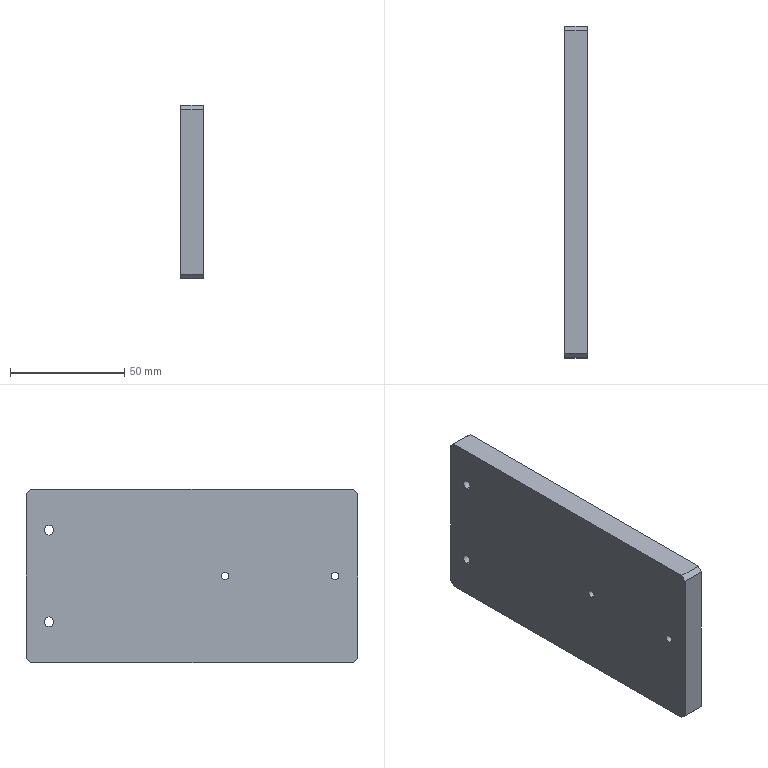Part | SolidWorks | features HoleWzd 2, Chamfer 1, Extrusion 1 | 1 solid | 18 faces | box 10 x 145 x 76 mm | volume 109672 mm3 | plane 10 | cylinder 8 | commonest cylinder face diameters 3.3 x4 4.2 x4
STEP:
#1=CARTESIAN_POINT('',(10.,-14.5,-1.65));
#2=VERTEX_POINT('',#1);
#3=CARTESIAN_POINT('',(10.,-14.5,1.65));
#4=VERTEX_POINT('',#3);
#5=CARTESIAN_POINT('',(10.,-14.5,0.));
#6=DIRECTION('',(-1.,0.,0.));
#7=DIRECTION('',(0.,0.,1.));
#8=AXIS2_PLACEMENT_3D('',#5,#6,#7);
#9=CIRCLE('',#8,1.65);
#10=EDGE_CURVE('',#2,#4,#9,.T.);
#11=ORIENTED_EDGE('',*,*,#10,.F.);
#12=CARTESIAN_POINT('',(0.,-14.5,-1.65));
#13=VERTEX_POINT('',#12);
#14=CARTESIAN_POINT('',(0.,-14.5,-1.65));
#15=DIRECTION('',(-1.,0.,0.));
#16=VECTOR('',#15,1000.);
#17=LINE('',#14,#16);
#18=EDGE_CURVE('',#2,#13,#17,.T.);
#19=ORIENTED_EDGE('',*,*,#18,.T.);
#20=CARTESIAN_POINT('',(0.,-14.5,1.65));
#21=VERTEX_POINT('',#20);
#22=CARTESIAN_POINT('',(0.,-14.5,0.));
#23=DIRECTION('',(-1.,0.,0.));
#24=DIRECTION('',(0.,0.,1.));
#25=AXIS2_PLACEMENT_3D('',#22,#23,#24);
#26=CIRCLE('',#25,1.65);
#27=EDGE_CURVE('',#13,#21,#26,.T.);
#28=ORIENTED_EDGE('',*,*,#27,.T.);
#29=CARTESIAN_POINT('',(0.,-14.5,1.65));
#30=DIRECTION('',(-1.,0.,0.));
#31=VECTOR('',#30,1000.);
#32=LINE('',#29,#31);
#33=EDGE_CURVE('',#4,#21,#32,.T.);
#34=ORIENTED_EDGE('',*,*,#33,.F.);
#35=EDGE_LOOP('',(#11,#19,#28,#34));
#36=FACE_OUTER_BOUND('',#35,.T.);
#37=CARTESIAN_POINT('',(0.,-14.5,0.));
#38=DIRECTION('',(-1.,0.,0.));
#39=DIRECTION('',(0.,0.,1.));
#40=AXIS2_PLACEMENT_3D('',#37,#38,#39);
#41=CYLINDRICAL_SURFACE('',#40,1.65);
#42=ADVANCED_FACE('',(#36),#41,.F.);
#43=CARTESIAN_POINT('',(10.,-62.5,-1.65));
#44=VERTEX_POINT('',#43);
#45=CARTESIAN_POINT('',(10.,-62.5,1.65));
#46=VERTEX_POINT('',#45);
#47=CARTESIAN_POINT('',(10.,-62.5,0.));
#48=DIRECTION('',(-1.,0.,0.));
#49=DIRECTION('',(0.,0.,1.));
#50=AXIS2_PLACEMENT_3D('',#47,#48,#49);
#51=CIRCLE('',#50,1.65);
#52=EDGE_CURVE('',#44,#46,#51,.T.);
#53=ORIENTED_EDGE('',*,*,#52,.F.);
#54=CARTESIAN_POINT('',(0.,-62.5,-1.65));
#55=VERTEX_POINT('',#54);
#56=CARTESIAN_POINT('',(0.,-62.5,-1.65));
#57=DIRECTION('',(-1.,0.,0.));
#58=VECTOR('',#57,1000.);
#59=LINE('',#56,#58);
#60=EDGE_CURVE('',#44,#55,#59,.T.);
#61=ORIENTED_EDGE('',*,*,#60,.T.);
#62=CARTESIAN_POINT('',(0.,-62.5,1.65));
#63=VERTEX_POINT('',#62);
#64=CARTESIAN_POINT('',(0.,-62.5,0.));
#65=DIRECTION('',(-1.,0.,0.));
#66=DIRECTION('',(0.,0.,1.));
#67=AXIS2_PLACEMENT_3D('',#64,#65,#66);
#68=CIRCLE('',#67,1.65);
#69=EDGE_CURVE('',#55,#63,#68,.T.);
#70=ORIENTED_EDGE('',*,*,#69,.T.);
#71=CARTESIAN_POINT('',(0.,-62.5,1.65));
#72=DIRECTION('',(-1.,0.,0.));
#73=VECTOR('',#72,1000.);
#74=LINE('',#71,#73);
#75=EDGE_CURVE('',#46,#63,#74,.T.);
#76=ORIENTED_EDGE('',*,*,#75,.F.);
#77=EDGE_LOOP('',(#53,#61,#70,#76));
#78=FACE_OUTER_BOUND('',#77,.T.);
#79=CARTESIAN_POINT('',(0.,-62.5,0.));
#80=DIRECTION('',(-1.,0.,0.));
#81=DIRECTION('',(0.,0.,1.));
#82=AXIS2_PLACEMENT_3D('',#79,#80,#81);
#83=CYLINDRICAL_SURFACE('',#82,1.65);
#84=ADVANCED_FACE('',(#78),#83,.F.);
#85=CARTESIAN_POINT('',(10.,62.5,17.9));
#86=VERTEX_POINT('',#85);
#87=CARTESIAN_POINT('',(10.,62.5,22.1));
#88=VERTEX_POINT('',#87);
#89=CARTESIAN_POINT('',(10.,62.5,20.));
#90=DIRECTION('',(-1.,0.,0.));
#91=DIRECTION('',(0.,0.,1.));
#92=AXIS2_PLACEMENT_3D('',#89,#90,#91);
#93=CIRCLE('',#92,2.1);
#94=EDGE_CURVE('',#86,#88,#93,.T.);
#95=ORIENTED_EDGE('',*,*,#94,.F.);
#96=CARTESIAN_POINT('',(0.,62.5,17.9));
#97=VERTEX_POINT('',#96);
#98=CARTESIAN_POINT('',(0.,62.5,17.9));
#99=DIRECTION('',(-1.,0.,0.));
#100=VECTOR('',#99,1000.);
#101=LINE('',#98,#100);
#102=EDGE_CURVE('',#86,#97,#101,.T.);
#103=ORIENTED_EDGE('',*,*,#102,.T.);
#104=CARTESIAN_POINT('',(0.,62.5,22.1));
#105=VERTEX_POINT('',#104);
#106=CARTESIAN_POINT('',(0.,62.5,20.));
#107=DIRECTION('',(-1.,0.,0.));
#108=DIRECTION('',(0.,0.,1.));
#109=AXIS2_PLACEMENT_3D('',#106,#107,#108);
#110=CIRCLE('',#109,2.1);
#111=EDGE_CURVE('',#97,#105,#110,.T.);
#112=ORIENTED_EDGE('',*,*,#111,.T.);
#113=CARTESIAN_POINT('',(0.,62.5,22.1));
#114=DIRECTION('',(-1.,0.,0.));
#115=VECTOR('',#114,1000.);
#116=LINE('',#113,#115);
#117=EDGE_CURVE('',#88,#105,#116,.T.);
#118=ORIENTED_EDGE('',*,*,#117,.F.);
#119=EDGE_LOOP('',(#95,#103,#112,#118));
#120=FACE_OUTER_BOUND('',#119,.T.);
#121=CARTESIAN_POINT('',(0.,62.5,20.));
#122=DIRECTION('',(-1.,0.,0.));
#123=DIRECTION('',(0.,0.,1.));
#124=AXIS2_PLACEMENT_3D('',#121,#122,#123);
#125=CYLINDRICAL_SURFACE('',#124,2.1);
#126=ADVANCED_FACE('',(#120),#125,.F.);
#127=CARTESIAN_POINT('',(10.,62.5,-22.1));
#128=VERTEX_POINT('',#127);
#129=CARTESIAN_POINT('',(10.,62.5,-17.9));
#130=VERTEX_POINT('',#129);
#131=CARTESIAN_POINT('',(10.,62.5,-20.));
#132=DIRECTION('',(-1.,0.,0.));
#133=DIRECTION('',(0.,0.,1.));
#134=AXIS2_PLACEMENT_3D('',#131,#132,#133);
#135=CIRCLE('',#134,2.1);
#136=EDGE_CURVE('',#128,#130,#135,.T.);
#137=ORIENTED_EDGE('',*,*,#136,.F.);
#138=CARTESIAN_POINT('',(0.,62.5,-22.1));
#139=VERTEX_POINT('',#138);
#140=CARTESIAN_POINT('',(0.,62.5,-22.1));
#141=DIRECTION('',(-1.,0.,0.));
#142=VECTOR('',#141,1000.);
#143=LINE('',#140,#142);
#144=EDGE_CURVE('',#128,#139,#143,.T.);
#145=ORIENTED_EDGE('',*,*,#144,.T.);
#146=CARTESIAN_POINT('',(0.,62.5,-17.9));
#147=VERTEX_POINT('',#146);
#148=CARTESIAN_POINT('',(0.,62.5,-20.));
#149=DIRECTION('',(-1.,0.,0.));
#150=DIRECTION('',(0.,0.,1.));
#151=AXIS2_PLACEMENT_3D('',#148,#149,#150);
#152=CIRCLE('',#151,2.1);
#153=EDGE_CURVE('',#139,#147,#152,.T.);
#154=ORIENTED_EDGE('',*,*,#153,.T.);
#155=CARTESIAN_POINT('',(0.,62.5,-17.9));
#156=DIRECTION('',(-1.,0.,0.));
#157=VECTOR('',#156,1000.);
#158=LINE('',#155,#157);
#159=EDGE_CURVE('',#130,#147,#158,.T.);
#160=ORIENTED_EDGE('',*,*,#159,.F.);
#161=EDGE_LOOP('',(#137,#145,#154,#160));
#162=FACE_OUTER_BOUND('',#161,.T.);
#163=CARTESIAN_POINT('',(0.,62.5,-20.));
#164=DIRECTION('',(-1.,0.,0.));
#165=DIRECTION('',(0.,0.,1.));
#166=AXIS2_PLACEMENT_3D('',#163,#164,#165);
#167=CYLINDRICAL_SURFACE('',#166,2.1);
#168=ADVANCED_FACE('',(#162),#167,.F.);
#169=CARTESIAN_POINT('',(10.,-70.5,-38.));
#170=VERTEX_POINT('',#169);
#171=CARTESIAN_POINT('',(10.,70.5,-38.));
#172=VERTEX_POINT('',#171);
#173=CARTESIAN_POINT('',(10.,72.5,-38.));
#174=DIRECTION('',(0.,1.,0.));
#175=VECTOR('',#174,1000.);
#176=LINE('',#173,#175);
#177=EDGE_CURVE('',#170,#172,#176,.T.);
#178=ORIENTED_EDGE('',*,*,#177,.F.);
#179=CARTESIAN_POINT('',(0.,-70.5,-38.));
#180=VERTEX_POINT('',#179);
#181=CARTESIAN_POINT('',(10.,-70.5,-38.));
#182=DIRECTION('',(-1.,0.,0.));
#183=VECTOR('',#182,1000.);
#184=LINE('',#181,#183);
#185=EDGE_CURVE('',#170,#180,#184,.T.);
#186=ORIENTED_EDGE('',*,*,#185,.T.);
#187=CARTESIAN_POINT('',(0.,70.5,-38.));
#188=VERTEX_POINT('',#187);
#189=CARTESIAN_POINT('',(0.,72.5,-38.));
#190=DIRECTION('',(0.,1.,0.));
#191=VECTOR('',#190,1000.);
#192=LINE('',#189,#191);
#193=EDGE_CURVE('',#180,#188,#192,.T.);
#194=ORIENTED_EDGE('',*,*,#193,.T.);
#195=CARTESIAN_POINT('',(10.,70.5,-38.));
#196=DIRECTION('',(1.,0.,0.));
#197=VECTOR('',#196,1000.);
#198=LINE('',#195,#197);
#199=EDGE_CURVE('',#188,#172,#198,.T.);
#200=ORIENTED_EDGE('',*,*,#199,.T.);
#201=EDGE_LOOP('',(#178,#186,#194,#200));
#202=FACE_OUTER_BOUND('',#201,.T.);
#203=CARTESIAN_POINT('',(10.,72.5,-38.));
#204=DIRECTION('',(0.,0.,1.));
#205=DIRECTION('',(0.,-1.,0.));
#206=AXIS2_PLACEMENT_3D('',#203,#204,#205);
#207=PLANE('',#206);
#208=ADVANCED_FACE('',(#202),#207,.F.);
#209=CARTESIAN_POINT('',(0.,72.5,-36.));
#210=VERTEX_POINT('',#209);
#211=CARTESIAN_POINT('',(0.,72.5,36.));
#212=VERTEX_POINT('',#211);
#213=CARTESIAN_POINT('',(0.,72.5,38.));
#214=DIRECTION('',(0.,0.,1.));
#215=VECTOR('',#214,1000.);
#216=LINE('',#213,#215);
#217=EDGE_CURVE('',#210,#212,#216,.T.);
#218=ORIENTED_EDGE('',*,*,#217,.T.);
#219=CARTESIAN_POINT('',(10.,72.5,36.));
#220=VERTEX_POINT('',#219);
#221=CARTESIAN_POINT('',(10.,72.5,36.));
#222=DIRECTION('',(1.,0.,0.));
#223=VECTOR('',#222,1000.);
#224=LINE('',#221,#223);
#225=EDGE_CURVE('',#212,#220,#224,.T.);
#226=ORIENTED_EDGE('',*,*,#225,.T.);
#227=CARTESIAN_POINT('',(10.,72.5,-36.));
#228=VERTEX_POINT('',#227);
#229=CARTESIAN_POINT('',(10.,72.5,38.));
#230=DIRECTION('',(0.,0.,1.));
#231=VECTOR('',#230,1000.);
#232=LINE('',#229,#231);
#233=EDGE_CURVE('',#228,#220,#232,.T.);
#234=ORIENTED_EDGE('',*,*,#233,.F.);
#235=CARTESIAN_POINT('',(10.,72.5,-36.));
#236=DIRECTION('',(-1.,0.,0.));
#237=VECTOR('',#236,1000.);
#238=LINE('',#235,#237);
#239=EDGE_CURVE('',#228,#210,#238,.T.);
#240=ORIENTED_EDGE('',*,*,#239,.T.);
#241=EDGE_LOOP('',(#218,#226,#234,#240));
#242=FACE_OUTER_BOUND('',#241,.T.);
#243=CARTESIAN_POINT('',(10.,72.5,38.));
#244=DIRECTION('',(0.,-1.,0.));
#245=DIRECTION('',(0.,0.,-1.));
#246=AXIS2_PLACEMENT_3D('',#243,#244,#245);
#247=PLANE('',#246);
#248=ADVANCED_FACE('',(#242),#247,.F.);
#249=CARTESIAN_POINT('',(0.,70.5,38.));
#250=VERTEX_POINT('',#249);
#251=CARTESIAN_POINT('',(0.,-70.5,38.));
#252=VERTEX_POINT('',#251);
#253=CARTESIAN_POINT('',(0.,72.5,38.));
#254=DIRECTION('',(0.,-1.,0.));
#255=VECTOR('',#254,1000.);
#256=LINE('',#253,#255);
#257=EDGE_CURVE('',#250,#252,#256,.T.);
#258=ORIENTED_EDGE('',*,*,#257,.T.);
#259=CARTESIAN_POINT('',(10.,-70.5,38.));
#260=VERTEX_POINT('',#259);
#261=CARTESIAN_POINT('',(10.,-70.5,38.));
#262=DIRECTION('',(1.,0.,0.));
#263=VECTOR('',#262,1000.);
#264=LINE('',#261,#263);
#265=EDGE_CURVE('',#252,#260,#264,.T.);
#266=ORIENTED_EDGE('',*,*,#265,.T.);
#267=CARTESIAN_POINT('',(10.,70.5,38.));
#268=VERTEX_POINT('',#267);
#269=CARTESIAN_POINT('',(10.,72.5,38.));
#270=DIRECTION('',(0.,-1.,0.));
#271=VECTOR('',#270,1000.);
#272=LINE('',#269,#271);
#273=EDGE_CURVE('',#268,#260,#272,.T.);
#274=ORIENTED_EDGE('',*,*,#273,.F.);
#275=CARTESIAN_POINT('',(10.,70.5,38.));
#276=DIRECTION('',(-1.,0.,0.));
#277=VECTOR('',#276,1000.);
#278=LINE('',#275,#277);
#279=EDGE_CURVE('',#268,#250,#278,.T.);
#280=ORIENTED_EDGE('',*,*,#279,.T.);
#281=EDGE_LOOP('',(#258,#266,#274,#280));
#282=FACE_OUTER_BOUND('',#281,.T.);
#283=CARTESIAN_POINT('',(10.,72.5,38.));
#284=DIRECTION('',(0.,0.,-1.));
#285=DIRECTION('',(0.,1.,0.));
#286=AXIS2_PLACEMENT_3D('',#283,#284,#285);
#287=PLANE('',#286);
#288=ADVANCED_FACE('',(#282),#287,.F.);
#289=CARTESIAN_POINT('',(0.,-72.5,36.));
#290=VERTEX_POINT('',#289);
#291=CARTESIAN_POINT('',(0.,-72.5,-36.));
#292=VERTEX_POINT('',#291);
#293=CARTESIAN_POINT('',(0.,-72.5,38.));
#294=DIRECTION('',(0.,0.,-1.));
#295=VECTOR('',#294,1000.);
#296=LINE('',#293,#295);
#297=EDGE_CURVE('',#290,#292,#296,.T.);
#298=ORIENTED_EDGE('',*,*,#297,.T.);
#299=CARTESIAN_POINT('',(10.,-72.5,-36.));
#300=VERTEX_POINT('',#299);
#301=CARTESIAN_POINT('',(10.,-72.5,-36.));
#302=DIRECTION('',(1.,0.,0.));
#303=VECTOR('',#302,1000.);
#304=LINE('',#301,#303);
#305=EDGE_CURVE('',#292,#300,#304,.T.);
#306=ORIENTED_EDGE('',*,*,#305,.T.);
#307=CARTESIAN_POINT('',(10.,-72.5,36.));
#308=VERTEX_POINT('',#307);
#309=CARTESIAN_POINT('',(10.,-72.5,38.));
#310=DIRECTION('',(0.,0.,-1.));
#311=VECTOR('',#310,1000.);
#312=LINE('',#309,#311);
#313=EDGE_CURVE('',#308,#300,#312,.T.);
#314=ORIENTED_EDGE('',*,*,#313,.F.);
#315=CARTESIAN_POINT('',(10.,-72.5,36.));
#316=DIRECTION('',(-1.,0.,0.));
#317=VECTOR('',#316,1000.);
#318=LINE('',#315,#317);
#319=EDGE_CURVE('',#308,#290,#318,.T.);
#320=ORIENTED_EDGE('',*,*,#319,.T.);
#321=EDGE_LOOP('',(#298,#306,#314,#320));
#322=FACE_OUTER_BOUND('',#321,.T.);
#323=CARTESIAN_POINT('',(10.,-72.5,38.));
#324=DIRECTION('',(0.,1.,0.));
#325=DIRECTION('',(0.,0.,1.));
#326=AXIS2_PLACEMENT_3D('',#323,#324,#325);
#327=PLANE('',#326);
#328=ADVANCED_FACE('',(#322),#327,.F.);
#329=CARTESIAN_POINT('',(10.,-14.5,0.));
#330=DIRECTION('',(-1.,0.,0.));
#331=DIRECTION('',(0.,0.,1.));
#332=AXIS2_PLACEMENT_3D('',#329,#330,#331);
#333=CIRCLE('',#332,1.65);
#334=EDGE_CURVE('',#4,#2,#333,.T.);
#335=ORIENTED_EDGE('',*,*,#334,.T.);
#336=ORIENTED_EDGE('',*,*,#10,.T.);
#337=EDGE_LOOP('',(#335,#336));
#338=FACE_BOUND('',#337,.T.);
#339=CARTESIAN_POINT('',(10.,-62.5,0.));
#340=DIRECTION('',(-1.,0.,0.));
#341=DIRECTION('',(0.,0.,1.));
#342=AXIS2_PLACEMENT_3D('',#339,#340,#341);
#343=CIRCLE('',#342,1.65);
#344=EDGE_CURVE('',#46,#44,#343,.T.);
#345=ORIENTED_EDGE('',*,*,#344,.T.);
#346=ORIENTED_EDGE('',*,*,#52,.T.);
#347=EDGE_LOOP('',(#345,#346));
#348=FACE_BOUND('',#347,.T.);
#349=CARTESIAN_POINT('',(10.,62.5,20.));
#350=DIRECTION('',(-1.,0.,0.));
#351=DIRECTION('',(0.,0.,1.));
#352=AXIS2_PLACEMENT_3D('',#349,#350,#351);
#353=CIRCLE('',#352,2.1);
#354=EDGE_CURVE('',#88,#86,#353,.T.);
#355=ORIENTED_EDGE('',*,*,#354,.T.);
#356=ORIENTED_EDGE('',*,*,#94,.T.);
#357=EDGE_LOOP('',(#355,#356));
#358=FACE_BOUND('',#357,.T.);
#359=CARTESIAN_POINT('',(10.,62.5,-20.));
#360=DIRECTION('',(-1.,0.,0.));
#361=DIRECTION('',(0.,0.,1.));
#362=AXIS2_PLACEMENT_3D('',#359,#360,#361);
#363=CIRCLE('',#362,2.1);
#364=EDGE_CURVE('',#130,#128,#363,.T.);
#365=ORIENTED_EDGE('',*,*,#364,.T.);
#366=ORIENTED_EDGE('',*,*,#136,.T.);
#367=EDGE_LOOP('',(#365,#366));
#368=FACE_BOUND('',#367,.T.);
#369=ORIENTED_EDGE('',*,*,#313,.T.);
#370=CARTESIAN_POINT('',(10.,-54.25,-54.25));
#371=DIRECTION('',(0.,0.7071,-0.7071));
#372=VECTOR('',#371,1000.);
#373=LINE('',#370,#372);
#374=EDGE_CURVE('',#300,#170,#373,.T.);
#375=ORIENTED_EDGE('',*,*,#374,.T.);
#376=ORIENTED_EDGE('',*,*,#177,.T.);
#377=CARTESIAN_POINT('',(10.,54.25,-54.25));
#378=DIRECTION('',(0.,0.7071,0.7071));
#379=VECTOR('',#378,1000.);
#380=LINE('',#377,#379);
#381=EDGE_CURVE('',#172,#228,#380,.T.);
#382=ORIENTED_EDGE('',*,*,#381,.T.);
#383=ORIENTED_EDGE('',*,*,#233,.T.);
#384=CARTESIAN_POINT('',(10.,54.25,54.25));
#385=DIRECTION('',(0.,-0.7071,0.7071));
#386=VECTOR('',#385,1000.);
#387=LINE('',#384,#386);
#388=EDGE_CURVE('',#220,#268,#387,.T.);
#389=ORIENTED_EDGE('',*,*,#388,.T.);
#390=ORIENTED_EDGE('',*,*,#273,.T.);
#391=CARTESIAN_POINT('',(10.,-54.25,54.25));
#392=DIRECTION('',(0.,-0.7071,-0.7071));
#393=VECTOR('',#392,1000.);
#394=LINE('',#391,#393);
#395=EDGE_CURVE('',#260,#308,#394,.T.);
#396=ORIENTED_EDGE('',*,*,#395,.T.);
#397=EDGE_LOOP('',(#369,#375,#376,#382,#383,#389,#390,#396));
#398=FACE_OUTER_BOUND('',#397,.T.);
#399=CARTESIAN_POINT('',(10.,0.,0.));
#400=DIRECTION('',(1.,0.,0.));
#401=DIRECTION('',(0.,0.,-1.));
#402=AXIS2_PLACEMENT_3D('',#399,#400,#401);
#403=PLANE('',#402);
#404=ADVANCED_FACE('',(#338,#348,#358,#368,#398),#403,.T.);
#405=CARTESIAN_POINT('',(0.,-14.5,0.));
#406=DIRECTION('',(-1.,0.,0.));
#407=DIRECTION('',(0.,0.,1.));
#408=AXIS2_PLACEMENT_3D('',#405,#406,#407);
#409=CIRCLE('',#408,1.65);
#410=EDGE_CURVE('',#21,#13,#409,.T.);
#411=ORIENTED_EDGE('',*,*,#410,.F.);
#412=ORIENTED_EDGE('',*,*,#27,.F.);
#413=EDGE_LOOP('',(#411,#412));
#414=FACE_BOUND('',#413,.T.);
#415=CARTESIAN_POINT('',(0.,-62.5,0.));
#416=DIRECTION('',(-1.,0.,0.));
#417=DIRECTION('',(0.,0.,1.));
#418=AXIS2_PLACEMENT_3D('',#415,#416,#417);
#419=CIRCLE('',#418,1.65);
#420=EDGE_CURVE('',#63,#55,#419,.T.);
#421=ORIENTED_EDGE('',*,*,#420,.F.);
#422=ORIENTED_EDGE('',*,*,#69,.F.);
#423=EDGE_LOOP('',(#421,#422));
#424=FACE_BOUND('',#423,.T.);
#425=CARTESIAN_POINT('',(0.,62.5,20.));
#426=DIRECTION('',(-1.,0.,0.));
#427=DIRECTION('',(0.,0.,1.));
#428=AXIS2_PLACEMENT_3D('',#425,#426,#427);
#429=CIRCLE('',#428,2.1);
#430=EDGE_CURVE('',#105,#97,#429,.T.);
#431=ORIENTED_EDGE('',*,*,#430,.F.);
#432=ORIENTED_EDGE('',*,*,#111,.F.);
#433=EDGE_LOOP('',(#431,#432));
#434=FACE_BOUND('',#433,.T.);
#435=CARTESIAN_POINT('',(0.,62.5,-20.));
#436=DIRECTION('',(-1.,0.,0.));
#437=DIRECTION('',(0.,0.,1.));
#438=AXIS2_PLACEMENT_3D('',#435,#436,#437);
#439=CIRCLE('',#438,2.1);
#440=EDGE_CURVE('',#147,#139,#439,.T.);
#441=ORIENTED_EDGE('',*,*,#440,.F.);
#442=ORIENTED_EDGE('',*,*,#153,.F.);
#443=EDGE_LOOP('',(#441,#442));
#444=FACE_BOUND('',#443,.T.);
#445=ORIENTED_EDGE('',*,*,#193,.F.);
#446=CARTESIAN_POINT('',(0.,-70.5,-38.));
#447=DIRECTION('',(0.,-0.7071,0.7071));
#448=VECTOR('',#447,1000.);
#449=LINE('',#446,#448);
#450=EDGE_CURVE('',#180,#292,#449,.T.);
#451=ORIENTED_EDGE('',*,*,#450,.T.);
#452=ORIENTED_EDGE('',*,*,#297,.F.);
#453=CARTESIAN_POINT('',(0.,-72.5,36.));
#454=DIRECTION('',(0.,0.7071,0.7071));
#455=VECTOR('',#454,1000.);
#456=LINE('',#453,#455);
#457=EDGE_CURVE('',#290,#252,#456,.T.);
#458=ORIENTED_EDGE('',*,*,#457,.T.);
#459=ORIENTED_EDGE('',*,*,#257,.F.);
#460=CARTESIAN_POINT('',(0.,70.5,38.));
#461=DIRECTION('',(0.,0.7071,-0.7071));
#462=VECTOR('',#461,1000.);
#463=LINE('',#460,#462);
#464=EDGE_CURVE('',#250,#212,#463,.T.);
#465=ORIENTED_EDGE('',*,*,#464,.T.);
#466=ORIENTED_EDGE('',*,*,#217,.F.);
#467=CARTESIAN_POINT('',(0.,72.5,-36.));
#468=DIRECTION('',(0.,-0.7071,-0.7071));
#469=VECTOR('',#468,1000.);
#470=LINE('',#467,#469);
#471=EDGE_CURVE('',#210,#188,#470,.T.);
#472=ORIENTED_EDGE('',*,*,#471,.T.);
#473=EDGE_LOOP('',(#445,#451,#452,#458,#459,#465,#466,#472));
#474=FACE_OUTER_BOUND('',#473,.T.);
#475=CARTESIAN_POINT('',(0.,0.,0.));
#476=DIRECTION('',(1.,0.,0.));
#477=DIRECTION('',(0.,0.,-1.));
#478=AXIS2_PLACEMENT_3D('',#475,#476,#477);
#479=PLANE('',#478);
#480=ADVANCED_FACE('',(#414,#424,#434,#444,#474),#479,.F.);
#481=ORIENTED_EDGE('',*,*,#144,.F.);
#482=ORIENTED_EDGE('',*,*,#364,.F.);
#483=ORIENTED_EDGE('',*,*,#159,.T.);
#484=ORIENTED_EDGE('',*,*,#440,.T.);
#485=EDGE_LOOP('',(#481,#482,#483,#484));
#486=FACE_OUTER_BOUND('',#485,.T.);
#487=CARTESIAN_POINT('',(0.,62.5,-20.));
#488=DIRECTION('',(-1.,0.,0.));
#489=DIRECTION('',(0.,0.,1.));
#490=AXIS2_PLACEMENT_3D('',#487,#488,#489);
#491=CYLINDRICAL_SURFACE('',#490,2.1);
#492=ADVANCED_FACE('',(#486),#491,.F.);
#493=ORIENTED_EDGE('',*,*,#102,.F.);
#494=ORIENTED_EDGE('',*,*,#354,.F.);
#495=ORIENTED_EDGE('',*,*,#117,.T.);
#496=ORIENTED_EDGE('',*,*,#430,.T.);
#497=EDGE_LOOP('',(#493,#494,#495,#496));
#498=FACE_OUTER_BOUND('',#497,.T.);
#499=CARTESIAN_POINT('',(0.,62.5,20.));
#500=DIRECTION('',(-1.,0.,0.));
#501=DIRECTION('',(0.,0.,1.));
#502=AXIS2_PLACEMENT_3D('',#499,#500,#501);
#503=CYLINDRICAL_SURFACE('',#502,2.1);
#504=ADVANCED_FACE('',(#498),#503,.F.);
#505=ORIENTED_EDGE('',*,*,#60,.F.);
#506=ORIENTED_EDGE('',*,*,#344,.F.);
#507=ORIENTED_EDGE('',*,*,#75,.T.);
#508=ORIENTED_EDGE('',*,*,#420,.T.);
#509=EDGE_LOOP('',(#505,#506,#507,#508));
#510=FACE_OUTER_BOUND('',#509,.T.);
#511=CARTESIAN_POINT('',(0.,-62.5,0.));
#512=DIRECTION('',(-1.,0.,0.));
#513=DIRECTION('',(0.,0.,1.));
#514=AXIS2_PLACEMENT_3D('',#511,#512,#513);
#515=CYLINDRICAL_SURFACE('',#514,1.65);
#516=ADVANCED_FACE('',(#510),#515,.F.);
#517=ORIENTED_EDGE('',*,*,#18,.F.);
#518=ORIENTED_EDGE('',*,*,#334,.F.);
#519=ORIENTED_EDGE('',*,*,#33,.T.);
#520=ORIENTED_EDGE('',*,*,#410,.T.);
#521=EDGE_LOOP('',(#517,#518,#519,#520));
#522=FACE_OUTER_BOUND('',#521,.T.);
#523=CARTESIAN_POINT('',(0.,-14.5,0.));
#524=DIRECTION('',(-1.,0.,0.));
#525=DIRECTION('',(0.,0.,1.));
#526=AXIS2_PLACEMENT_3D('',#523,#524,#525);
#527=CYLINDRICAL_SURFACE('',#526,1.65);
#528=ADVANCED_FACE('',(#522),#527,.F.);
#529=ORIENTED_EDGE('',*,*,#374,.F.);
#530=ORIENTED_EDGE('',*,*,#305,.F.);
#531=ORIENTED_EDGE('',*,*,#450,.F.);
#532=ORIENTED_EDGE('',*,*,#185,.F.);
#533=EDGE_LOOP('',(#529,#530,#531,#532));
#534=FACE_OUTER_BOUND('',#533,.T.);
#535=CARTESIAN_POINT('',(10.,-70.5,-38.));
#536=DIRECTION('',(0.,0.7071,0.7071));
#537=DIRECTION('',(-1.,0.,0.));
#538=AXIS2_PLACEMENT_3D('',#535,#536,#537);
#539=PLANE('',#538);
#540=ADVANCED_FACE('',(#534),#539,.F.);
#541=ORIENTED_EDGE('',*,*,#395,.F.);
#542=ORIENTED_EDGE('',*,*,#265,.F.);
#543=ORIENTED_EDGE('',*,*,#457,.F.);
#544=ORIENTED_EDGE('',*,*,#319,.F.);
#545=EDGE_LOOP('',(#541,#542,#543,#544));
#546=FACE_OUTER_BOUND('',#545,.T.);
#547=CARTESIAN_POINT('',(10.,-72.5,36.));
#548=DIRECTION('',(0.,0.7071,-0.7071));
#549=DIRECTION('',(-1.,0.,0.));
#550=AXIS2_PLACEMENT_3D('',#547,#548,#549);
#551=PLANE('',#550);
#552=ADVANCED_FACE('',(#546),#551,.F.);
#553=ORIENTED_EDGE('',*,*,#388,.F.);
#554=ORIENTED_EDGE('',*,*,#225,.F.);
#555=ORIENTED_EDGE('',*,*,#464,.F.);
#556=ORIENTED_EDGE('',*,*,#279,.F.);
#557=EDGE_LOOP('',(#553,#554,#555,#556));
#558=FACE_OUTER_BOUND('',#557,.T.);
#559=CARTESIAN_POINT('',(10.,70.5,38.));
#560=DIRECTION('',(0.,-0.7071,-0.7071));
#561=DIRECTION('',(-1.,0.,0.));
#562=AXIS2_PLACEMENT_3D('',#559,#560,#561);
#563=PLANE('',#562);
#564=ADVANCED_FACE('',(#558),#563,.F.);
#565=ORIENTED_EDGE('',*,*,#381,.F.);
#566=ORIENTED_EDGE('',*,*,#199,.F.);
#567=ORIENTED_EDGE('',*,*,#471,.F.);
#568=ORIENTED_EDGE('',*,*,#239,.F.);
#569=EDGE_LOOP('',(#565,#566,#567,#568));
#570=FACE_OUTER_BOUND('',#569,.T.);
#571=CARTESIAN_POINT('',(10.,72.5,-36.));
#572=DIRECTION('',(0.,-0.7071,0.7071));
#573=DIRECTION('',(-1.,0.,0.));
#574=AXIS2_PLACEMENT_3D('',#571,#572,#573);
#575=PLANE('',#574);
#576=ADVANCED_FACE('',(#570),#575,.F.);
#577=CLOSED_SHELL('',(#42,#84,#126,#168,#208,#248,#288,#328,#404,#480,#492,#504,#516,#528,#540,#552,#564,#576));
#578=MANIFOLD_SOLID_BREP('',#577);
#579=CARTESIAN_POINT('',(0.,0.,0.));
#580=DIRECTION('',(0.,0.,1.));
#581=DIRECTION('',(1.,0.,0.));
#582=AXIS2_PLACEMENT_3D('',#579,#580,#581);
#583=(LENGTH_UNIT()NAMED_UNIT(*)SI_UNIT(.MILLI.,.METRE.));
#584=UNCERTAINTY_MEASURE_WITH_UNIT(LENGTH_MEASURE(0.00001),#583,'','');
#585=(NAMED_UNIT(*)PLANE_ANGLE_UNIT()SI_UNIT($,.RADIAN.));
#586=(NAMED_UNIT(*)SI_UNIT($,.STERADIAN.)SOLID_ANGLE_UNIT());
#587=(GEOMETRIC_REPRESENTATION_CONTEXT(3)GLOBAL_UNCERTAINTY_ASSIGNED_CONTEXT((#584))GLOBAL_UNIT_ASSIGNED_CONTEXT((#583,#585,#586))REPRESENTATION_CONTEXT('',''));
#588=ADVANCED_BREP_SHAPE_REPRESENTATION('',(#578,#582),#587);